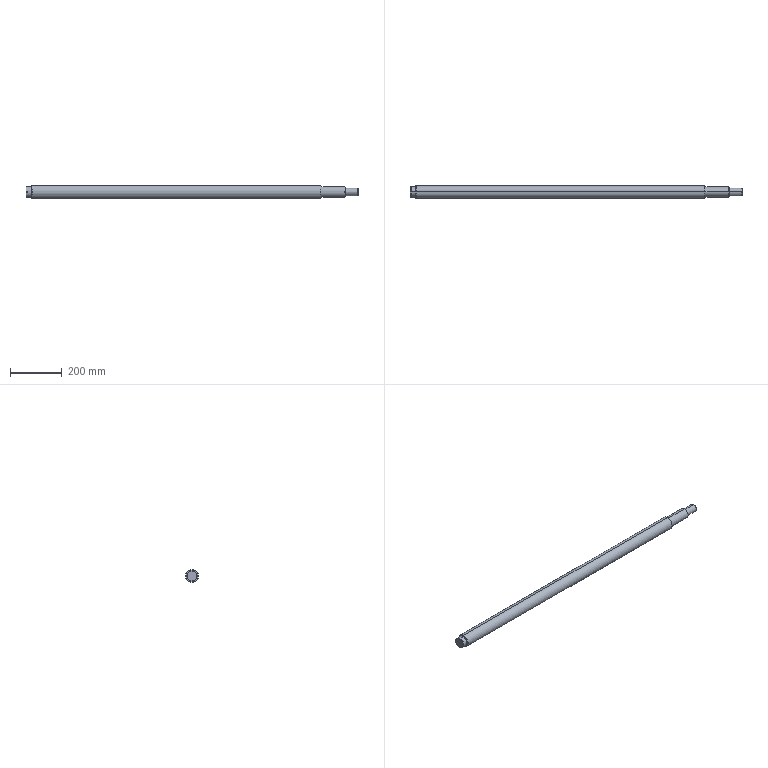Part | SolidWorks | features RefAxis 6, 3DProfileFeature 2, ICE 1, LockFeature 1, Revolution 1 | 1 solid | 36 faces | box 1281 x 50 x 50 mm | volume 2368676 mm3 | cylinder 14 | cone 10 | plane 10 | torus 2 | commonest cylinder face diameters 40 x6 8 x2 30 x2 38 x2 50 x2
STEP:
#1=CARTESIAN_POINT('',(0.,0.,19.));
#2=VERTEX_POINT('',#1);
#3=CARTESIAN_POINT('',(0.,0.,-19.));
#4=VERTEX_POINT('',#3);
#5=CARTESIAN_POINT('',(0.,0.,0.));
#6=DIRECTION('',(-1.,0.,0.));
#7=DIRECTION('',(0.,0.,1.));
#8=AXIS2_PLACEMENT_3D('',#5,#6,#7);
#9=CIRCLE('',#8,19.);
#10=EDGE_CURVE('',#2,#4,#9,.T.);
#11=ORIENTED_EDGE('',*,*,#10,.F.);
#12=CARTESIAN_POINT('',(1.,0.,20.));
#13=VERTEX_POINT('',#12);
#14=CARTESIAN_POINT('',(1.,0.,20.));
#15=DIRECTION('',(0.7071,0.,0.7071));
#16=VECTOR('',#15,1000.);
#17=LINE('',#14,#16);
#18=EDGE_CURVE('',#2,#13,#17,.T.);
#19=ORIENTED_EDGE('',*,*,#18,.T.);
#20=CARTESIAN_POINT('',(1.,0.,-20.));
#21=VERTEX_POINT('',#20);
#22=CARTESIAN_POINT('',(1.,0.,0.));
#23=DIRECTION('',(-1.,0.,0.));
#24=DIRECTION('',(0.,0.,1.));
#25=AXIS2_PLACEMENT_3D('',#22,#23,#24);
#26=CIRCLE('',#25,20.);
#27=EDGE_CURVE('',#13,#21,#26,.T.);
#28=ORIENTED_EDGE('',*,*,#27,.T.);
#29=CARTESIAN_POINT('',(1.,0.,-20.));
#30=DIRECTION('',(0.7071,0.,-0.7071));
#31=VECTOR('',#30,1000.);
#32=LINE('',#29,#31);
#33=EDGE_CURVE('',#4,#21,#32,.T.);
#34=ORIENTED_EDGE('',*,*,#33,.F.);
#35=EDGE_LOOP('',(#11,#19,#28,#34));
#36=FACE_OUTER_BOUND('',#35,.T.);
#37=CARTESIAN_POINT('',(1.,0.,0.));
#38=DIRECTION('',(1.,0.,0.));
#39=DIRECTION('',(0.,0.,-1.));
#40=AXIS2_PLACEMENT_3D('',#37,#38,#39);
#41=CONICAL_SURFACE('',#40,20.,0.7854);
#42=ADVANCED_FACE('',(#36),#41,.T.);
#43=CARTESIAN_POINT('',(3.05,0.,20.));
#44=VERTEX_POINT('',#43);
#45=CARTESIAN_POINT('',(3.05,0.,-20.));
#46=VERTEX_POINT('',#45);
#47=CARTESIAN_POINT('',(3.05,0.,0.));
#48=DIRECTION('',(-1.,0.,0.));
#49=DIRECTION('',(0.,0.,1.));
#50=AXIS2_PLACEMENT_3D('',#47,#48,#49);
#51=CIRCLE('',#50,20.);
#52=EDGE_CURVE('',#44,#46,#51,.T.);
#53=ORIENTED_EDGE('',*,*,#52,.T.);
#54=CARTESIAN_POINT('',(1281.,0.,-20.));
#55=DIRECTION('',(-1.,0.,0.));
#56=VECTOR('',#55,1000.);
#57=LINE('',#54,#56);
#58=EDGE_CURVE('',#46,#21,#57,.T.);
#59=ORIENTED_EDGE('',*,*,#58,.T.);
#60=ORIENTED_EDGE('',*,*,#27,.F.);
#61=CARTESIAN_POINT('',(1281.,0.,20.));
#62=DIRECTION('',(-1.,0.,0.));
#63=VECTOR('',#62,1000.);
#64=LINE('',#61,#63);
#65=EDGE_CURVE('',#44,#13,#64,.T.);
#66=ORIENTED_EDGE('',*,*,#65,.F.);
#67=EDGE_LOOP('',(#53,#59,#60,#66));
#68=FACE_OUTER_BOUND('',#67,.T.);
#69=CARTESIAN_POINT('',(1281.,0.,0.));
#70=DIRECTION('',(-1.,0.,0.));
#71=DIRECTION('',(0.,0.,1.));
#72=AXIS2_PLACEMENT_3D('',#69,#70,#71);
#73=CYLINDRICAL_SURFACE('',#72,20.);
#74=ADVANCED_FACE('',(#68),#73,.T.);
#75=CARTESIAN_POINT('',(5.,0.,19.));
#76=VERTEX_POINT('',#75);
#77=CARTESIAN_POINT('',(5.,0.,-19.));
#78=VERTEX_POINT('',#77);
#79=CARTESIAN_POINT('',(5.,0.,0.));
#80=DIRECTION('',(-1.,0.,0.));
#81=DIRECTION('',(0.,0.,1.));
#82=AXIS2_PLACEMENT_3D('',#79,#80,#81);
#83=CIRCLE('',#82,19.);
#84=EDGE_CURVE('',#76,#78,#83,.T.);
#85=ORIENTED_EDGE('',*,*,#84,.T.);
#86=CARTESIAN_POINT('',(3.05,0.,-19.));
#87=VERTEX_POINT('',#86);
#88=CARTESIAN_POINT('',(1281.,0.,-19.));
#89=DIRECTION('',(-1.,0.,0.));
#90=VECTOR('',#89,1000.);
#91=LINE('',#88,#90);
#92=EDGE_CURVE('',#78,#87,#91,.T.);
#93=ORIENTED_EDGE('',*,*,#92,.T.);
#94=CARTESIAN_POINT('',(3.05,0.,19.));
#95=VERTEX_POINT('',#94);
#96=CARTESIAN_POINT('',(3.05,0.,0.));
#97=DIRECTION('',(-1.,0.,0.));
#98=DIRECTION('',(0.,0.,1.));
#99=AXIS2_PLACEMENT_3D('',#96,#97,#98);
#100=CIRCLE('',#99,19.);
#101=EDGE_CURVE('',#95,#87,#100,.T.);
#102=ORIENTED_EDGE('',*,*,#101,.F.);
#103=CARTESIAN_POINT('',(1281.,0.,19.));
#104=DIRECTION('',(-1.,0.,0.));
#105=VECTOR('',#104,1000.);
#106=LINE('',#103,#105);
#107=EDGE_CURVE('',#76,#95,#106,.T.);
#108=ORIENTED_EDGE('',*,*,#107,.F.);
#109=EDGE_LOOP('',(#85,#93,#102,#108));
#110=FACE_OUTER_BOUND('',#109,.T.);
#111=CARTESIAN_POINT('',(1281.,0.,0.));
#112=DIRECTION('',(-1.,0.,0.));
#113=DIRECTION('',(0.,0.,1.));
#114=AXIS2_PLACEMENT_3D('',#111,#112,#113);
#115=CYLINDRICAL_SURFACE('',#114,19.);
#116=ADVANCED_FACE('',(#110),#115,.T.);
#117=CARTESIAN_POINT('',(22.75,0.,20.));
#118=VERTEX_POINT('',#117);
#119=CARTESIAN_POINT('',(22.75,0.,-20.));
#120=VERTEX_POINT('',#119);
#121=CARTESIAN_POINT('',(22.75,0.,0.));
#122=DIRECTION('',(-1.,0.,0.));
#123=DIRECTION('',(0.,0.,1.));
#124=AXIS2_PLACEMENT_3D('',#121,#122,#123);
#125=CIRCLE('',#124,20.);
#126=EDGE_CURVE('',#118,#120,#125,.T.);
#127=ORIENTED_EDGE('',*,*,#126,.T.);
#128=CARTESIAN_POINT('',(5.,0.,-20.));
#129=VERTEX_POINT('',#128);
#130=CARTESIAN_POINT('',(1281.,0.,-20.));
#131=DIRECTION('',(-1.,0.,0.));
#132=VECTOR('',#131,1000.);
#133=LINE('',#130,#132);
#134=EDGE_CURVE('',#120,#129,#133,.T.);
#135=ORIENTED_EDGE('',*,*,#134,.T.);
#136=CARTESIAN_POINT('',(5.,0.,20.));
#137=VERTEX_POINT('',#136);
#138=CARTESIAN_POINT('',(5.,0.,0.));
#139=DIRECTION('',(-1.,0.,0.));
#140=DIRECTION('',(0.,0.,1.));
#141=AXIS2_PLACEMENT_3D('',#138,#139,#140);
#142=CIRCLE('',#141,20.);
#143=EDGE_CURVE('',#137,#129,#142,.T.);
#144=ORIENTED_EDGE('',*,*,#143,.F.);
#145=CARTESIAN_POINT('',(1281.,0.,20.));
#146=DIRECTION('',(-1.,0.,0.));
#147=VECTOR('',#146,1000.);
#148=LINE('',#145,#147);
#149=EDGE_CURVE('',#118,#137,#148,.T.);
#150=ORIENTED_EDGE('',*,*,#149,.F.);
#151=EDGE_LOOP('',(#127,#135,#144,#150));
#152=FACE_OUTER_BOUND('',#151,.T.);
#153=CARTESIAN_POINT('',(1281.,0.,0.));
#154=DIRECTION('',(-1.,0.,0.));
#155=DIRECTION('',(0.,0.,1.));
#156=AXIS2_PLACEMENT_3D('',#153,#154,#155);
#157=CYLINDRICAL_SURFACE('',#156,20.);
#158=ADVANCED_FACE('',(#152),#157,.T.);
#159=CARTESIAN_POINT('',(22.75,0.,0.));
#160=DIRECTION('',(-1.,0.,0.));
#161=DIRECTION('',(0.,0.,1.));
#162=AXIS2_PLACEMENT_3D('',#159,#160,#161);
#163=CIRCLE('',#162,20.);
#164=EDGE_CURVE('',#120,#118,#163,.T.);
#165=ORIENTED_EDGE('',*,*,#164,.F.);
#166=CARTESIAN_POINT('',(23.,0.,-20.25));
#167=VERTEX_POINT('',#166);
#168=CARTESIAN_POINT('',(22.75,0.,-20.25));
#169=DIRECTION('',(0.,1.,0.));
#170=DIRECTION('',(0.,0.,1.));
#171=AXIS2_PLACEMENT_3D('',#168,#169,#170);
#172=CIRCLE('',#171,0.25);
#173=EDGE_CURVE('',#120,#167,#172,.T.);
#174=ORIENTED_EDGE('',*,*,#173,.T.);
#175=CARTESIAN_POINT('',(23.,0.,20.25));
#176=VERTEX_POINT('',#175);
#177=CARTESIAN_POINT('',(23.,0.,0.));
#178=DIRECTION('',(-1.,0.,0.));
#179=DIRECTION('',(0.,0.,1.));
#180=AXIS2_PLACEMENT_3D('',#177,#178,#179);
#181=CIRCLE('',#180,20.25);
#182=EDGE_CURVE('',#167,#176,#181,.T.);
#183=ORIENTED_EDGE('',*,*,#182,.T.);
#184=CARTESIAN_POINT('',(22.75,0.,20.25));
#185=DIRECTION('',(0.,-1.,0.));
#186=DIRECTION('',(0.,0.,-1.));
#187=AXIS2_PLACEMENT_3D('',#184,#185,#186);
#188=CIRCLE('',#187,0.25);
#189=EDGE_CURVE('',#118,#176,#188,.T.);
#190=ORIENTED_EDGE('',*,*,#189,.F.);
#191=EDGE_LOOP('',(#165,#174,#183,#190));
#192=FACE_OUTER_BOUND('',#191,.T.);
#193=CARTESIAN_POINT('',(22.75,0.,0.));
#194=DIRECTION('',(-1.,0.,0.));
#195=DIRECTION('',(0.,0.,1.));
#196=AXIS2_PLACEMENT_3D('',#193,#194,#195);
#197=TOROIDAL_SURFACE('',#196,20.25,0.25);
#198=ADVANCED_FACE('',(#192),#197,.F.);
#199=CARTESIAN_POINT('',(23.,0.,24.));
#200=VERTEX_POINT('',#199);
#201=CARTESIAN_POINT('',(23.,0.,-24.));
#202=VERTEX_POINT('',#201);
#203=CARTESIAN_POINT('',(23.,0.,0.));
#204=DIRECTION('',(-1.,0.,0.));
#205=DIRECTION('',(0.,0.,1.));
#206=AXIS2_PLACEMENT_3D('',#203,#204,#205);
#207=CIRCLE('',#206,24.);
#208=EDGE_CURVE('',#200,#202,#207,.T.);
#209=ORIENTED_EDGE('',*,*,#208,.F.);
#210=CARTESIAN_POINT('',(24.,0.,25.));
#211=VERTEX_POINT('',#210);
#212=CARTESIAN_POINT('',(24.,0.,25.));
#213=DIRECTION('',(0.7071,0.,0.7071));
#214=VECTOR('',#213,1000.);
#215=LINE('',#212,#214);
#216=EDGE_CURVE('',#200,#211,#215,.T.);
#217=ORIENTED_EDGE('',*,*,#216,.T.);
#218=CARTESIAN_POINT('',(24.,0.,-25.));
#219=VERTEX_POINT('',#218);
#220=CARTESIAN_POINT('',(24.,0.,0.));
#221=DIRECTION('',(-1.,0.,0.));
#222=DIRECTION('',(0.,0.,1.));
#223=AXIS2_PLACEMENT_3D('',#220,#221,#222);
#224=CIRCLE('',#223,25.);
#225=EDGE_CURVE('',#211,#219,#224,.T.);
#226=ORIENTED_EDGE('',*,*,#225,.T.);
#227=CARTESIAN_POINT('',(24.,0.,-25.));
#228=DIRECTION('',(0.7071,0.,-0.7071));
#229=VECTOR('',#228,1000.);
#230=LINE('',#227,#229);
#231=EDGE_CURVE('',#202,#219,#230,.T.);
#232=ORIENTED_EDGE('',*,*,#231,.F.);
#233=EDGE_LOOP('',(#209,#217,#226,#232));
#234=FACE_OUTER_BOUND('',#233,.T.);
#235=CARTESIAN_POINT('',(24.,0.,0.));
#236=DIRECTION('',(1.,0.,0.));
#237=DIRECTION('',(0.,0.,-1.));
#238=AXIS2_PLACEMENT_3D('',#235,#236,#237);
#239=CONICAL_SURFACE('',#238,25.,0.7854);
#240=ADVANCED_FACE('',(#234),#239,.T.);
#241=CARTESIAN_POINT('',(1137.,0.,25.));
#242=VERTEX_POINT('',#241);
#243=CARTESIAN_POINT('',(1137.,0.,-25.));
#244=VERTEX_POINT('',#243);
#245=CARTESIAN_POINT('',(1137.,0.,0.));
#246=DIRECTION('',(-1.,0.,0.));
#247=DIRECTION('',(0.,0.,1.));
#248=AXIS2_PLACEMENT_3D('',#245,#246,#247);
#249=CIRCLE('',#248,25.);
#250=EDGE_CURVE('',#242,#244,#249,.T.);
#251=ORIENTED_EDGE('',*,*,#250,.T.);
#252=CARTESIAN_POINT('',(1281.,0.,-25.));
#253=DIRECTION('',(-1.,0.,0.));
#254=VECTOR('',#253,1000.);
#255=LINE('',#252,#254);
#256=EDGE_CURVE('',#244,#219,#255,.T.);
#257=ORIENTED_EDGE('',*,*,#256,.T.);
#258=ORIENTED_EDGE('',*,*,#225,.F.);
#259=CARTESIAN_POINT('',(1281.,0.,25.));
#260=DIRECTION('',(-1.,0.,0.));
#261=VECTOR('',#260,1000.);
#262=LINE('',#259,#261);
#263=EDGE_CURVE('',#242,#211,#262,.T.);
#264=ORIENTED_EDGE('',*,*,#263,.F.);
#265=EDGE_LOOP('',(#251,#257,#258,#264));
#266=FACE_OUTER_BOUND('',#265,.T.);
#267=CARTESIAN_POINT('',(1281.,0.,0.));
#268=DIRECTION('',(-1.,0.,0.));
#269=DIRECTION('',(0.,0.,1.));
#270=AXIS2_PLACEMENT_3D('',#267,#268,#269);
#271=CYLINDRICAL_SURFACE('',#270,25.);
#272=ADVANCED_FACE('',(#266),#271,.T.);
#273=CARTESIAN_POINT('',(1138.,0.,24.));
#274=VERTEX_POINT('',#273);
#275=CARTESIAN_POINT('',(1138.,0.,-24.));
#276=VERTEX_POINT('',#275);
#277=CARTESIAN_POINT('',(1138.,0.,0.));
#278=DIRECTION('',(-1.,0.,0.));
#279=DIRECTION('',(0.,0.,1.));
#280=AXIS2_PLACEMENT_3D('',#277,#278,#279);
#281=CIRCLE('',#280,24.);
#282=EDGE_CURVE('',#274,#276,#281,.T.);
#283=ORIENTED_EDGE('',*,*,#282,.T.);
#284=CARTESIAN_POINT('',(1138.,0.,-24.));
#285=DIRECTION('',(-0.7071,0.,-0.7071));
#286=VECTOR('',#285,1000.);
#287=LINE('',#284,#286);
#288=EDGE_CURVE('',#276,#244,#287,.T.);
#289=ORIENTED_EDGE('',*,*,#288,.T.);
#290=ORIENTED_EDGE('',*,*,#250,.F.);
#291=CARTESIAN_POINT('',(1138.,0.,24.));
#292=DIRECTION('',(-0.7071,0.,0.7071));
#293=VECTOR('',#292,1000.);
#294=LINE('',#291,#293);
#295=EDGE_CURVE('',#274,#242,#294,.T.);
#296=ORIENTED_EDGE('',*,*,#295,.F.);
#297=EDGE_LOOP('',(#283,#289,#290,#296));
#298=FACE_OUTER_BOUND('',#297,.T.);
#299=CARTESIAN_POINT('',(1138.,0.,0.));
#300=DIRECTION('',(-1.,0.,0.));
#301=DIRECTION('',(0.,0.,1.));
#302=AXIS2_PLACEMENT_3D('',#299,#300,#301);
#303=CONICAL_SURFACE('',#302,24.,0.7854);
#304=ADVANCED_FACE('',(#298),#303,.T.);
#305=CARTESIAN_POINT('',(1230.,0.,20.));
#306=VERTEX_POINT('',#305);
#307=CARTESIAN_POINT('',(1230.,0.,-20.));
#308=VERTEX_POINT('',#307);
#309=CARTESIAN_POINT('',(1230.,0.,0.));
#310=DIRECTION('',(-1.,0.,0.));
#311=DIRECTION('',(0.,0.,1.));
#312=AXIS2_PLACEMENT_3D('',#309,#310,#311);
#313=CIRCLE('',#312,20.);
#314=EDGE_CURVE('',#306,#308,#313,.T.);
#315=ORIENTED_EDGE('',*,*,#314,.T.);
#316=CARTESIAN_POINT('',(1138.,0.,-20.));
#317=VERTEX_POINT('',#316);
#318=CARTESIAN_POINT('',(1281.,0.,-20.));
#319=DIRECTION('',(-1.,0.,0.));
#320=VECTOR('',#319,1000.);
#321=LINE('',#318,#320);
#322=EDGE_CURVE('',#308,#317,#321,.T.);
#323=ORIENTED_EDGE('',*,*,#322,.T.);
#324=CARTESIAN_POINT('',(1138.,0.,20.));
#325=VERTEX_POINT('',#324);
#326=CARTESIAN_POINT('',(1138.,0.,0.));
#327=DIRECTION('',(-1.,0.,0.));
#328=DIRECTION('',(0.,0.,1.));
#329=AXIS2_PLACEMENT_3D('',#326,#327,#328);
#330=CIRCLE('',#329,20.);
#331=EDGE_CURVE('',#325,#317,#330,.T.);
#332=ORIENTED_EDGE('',*,*,#331,.F.);
#333=CARTESIAN_POINT('',(1281.,0.,20.));
#334=DIRECTION('',(-1.,0.,0.));
#335=VECTOR('',#334,1000.);
#336=LINE('',#333,#335);
#337=EDGE_CURVE('',#306,#325,#336,.T.);
#338=ORIENTED_EDGE('',*,*,#337,.F.);
#339=EDGE_LOOP('',(#315,#323,#332,#338));
#340=FACE_OUTER_BOUND('',#339,.T.);
#341=CARTESIAN_POINT('',(1281.,0.,0.));
#342=DIRECTION('',(-1.,0.,0.));
#343=DIRECTION('',(0.,0.,1.));
#344=AXIS2_PLACEMENT_3D('',#341,#342,#343);
#345=CYLINDRICAL_SURFACE('',#344,20.);
#346=ADVANCED_FACE('',(#340),#345,.T.);
#347=CARTESIAN_POINT('',(1231.,0.,19.));
#348=VERTEX_POINT('',#347);
#349=CARTESIAN_POINT('',(1231.,0.,-19.));
#350=VERTEX_POINT('',#349);
#351=CARTESIAN_POINT('',(1231.,0.,0.));
#352=DIRECTION('',(-1.,0.,0.));
#353=DIRECTION('',(0.,0.,1.));
#354=AXIS2_PLACEMENT_3D('',#351,#352,#353);
#355=CIRCLE('',#354,19.);
#356=EDGE_CURVE('',#348,#350,#355,.T.);
#357=ORIENTED_EDGE('',*,*,#356,.T.);
#358=CARTESIAN_POINT('',(1231.,0.,-19.));
#359=DIRECTION('',(-0.7071,0.,-0.7071));
#360=VECTOR('',#359,1000.);
#361=LINE('',#358,#360);
#362=EDGE_CURVE('',#350,#308,#361,.T.);
#363=ORIENTED_EDGE('',*,*,#362,.T.);
#364=ORIENTED_EDGE('',*,*,#314,.F.);
#365=CARTESIAN_POINT('',(1231.,0.,19.));
#366=DIRECTION('',(-0.7071,0.,0.7071));
#367=VECTOR('',#366,1000.);
#368=LINE('',#365,#367);
#369=EDGE_CURVE('',#348,#306,#368,.T.);
#370=ORIENTED_EDGE('',*,*,#369,.F.);
#371=EDGE_LOOP('',(#357,#363,#364,#370));
#372=FACE_OUTER_BOUND('',#371,.T.);
#373=CARTESIAN_POINT('',(1231.,0.,0.));
#374=DIRECTION('',(-1.,0.,0.));
#375=DIRECTION('',(0.,0.,1.));
#376=AXIS2_PLACEMENT_3D('',#373,#374,#375);
#377=CONICAL_SURFACE('',#376,19.,0.7854);
#378=ADVANCED_FACE('',(#372),#377,.T.);
#379=CARTESIAN_POINT('',(1240.,14.457,-4.));
#380=VERTEX_POINT('',#379);
#381=CARTESIAN_POINT('',(1272.,14.457,-4.));
#382=VERTEX_POINT('',#381);
#383=CARTESIAN_POINT('',(1281.,14.457,-4.));
#384=DIRECTION('',(1.,0.,0.));
#385=VECTOR('',#384,1000.);
#386=LINE('',#383,#385);
#387=EDGE_CURVE('',#380,#382,#386,.T.);
#388=ORIENTED_EDGE('',*,*,#387,.T.);
#389=CARTESIAN_POINT('',(1272.,14.457,4.));
#390=VERTEX_POINT('',#389);
#391=CARTESIAN_POINT('',(1272.,14.457,-4.));
#392=CARTESIAN_POINT('',(1272.266,14.457,-4.));
#393=CARTESIAN_POINT('',(1272.526,14.464,-3.974));
#394=CARTESIAN_POINT('',(1273.039,14.492,-3.872));
#395=CARTESIAN_POINT('',(1273.294,14.513,-3.794));
#396=CARTESIAN_POINT('',(1273.777,14.564,-3.593));
#397=CARTESIAN_POINT('',(1274.007,14.594,-3.47));
#398=CARTESIAN_POINT('',(1274.44,14.66,-3.18));
#399=CARTESIAN_POINT('',(1274.645,14.696,-3.012));
#400=CARTESIAN_POINT('',(1275.012,14.766,-2.645));
#401=CARTESIAN_POINT('',(1275.177,14.801,-2.444));
#402=CARTESIAN_POINT('',(1275.47,14.867,-2.008));
#403=CARTESIAN_POINT('',(1275.593,14.896,-1.777));
#404=CARTESIAN_POINT('',(1275.793,14.946,-1.296));
#405=CARTESIAN_POINT('',(1275.871,14.966,-1.043));
#406=CARTESIAN_POINT('',(1275.974,14.993,-0.5261));
#407=CARTESIAN_POINT('',(1276.,15.,-0.2658));
#408=CARTESIAN_POINT('',(1276.,15.,0.2585));
#409=CARTESIAN_POINT('',(1275.974,14.993,0.5249));
#410=CARTESIAN_POINT('',(1275.872,14.966,1.039));
#411=CARTESIAN_POINT('',(1275.796,14.947,1.289));
#412=CARTESIAN_POINT('',(1275.494,14.872,2.017));
#413=CARTESIAN_POINT('',(1275.199,14.802,2.457));
#414=CARTESIAN_POINT('',(1274.645,14.696,3.012));
#415=CARTESIAN_POINT('',(1274.444,14.66,3.177));
#416=CARTESIAN_POINT('',(1274.012,14.595,3.467));
#417=CARTESIAN_POINT('',(1273.778,14.564,3.593));
#418=CARTESIAN_POINT('',(1273.296,14.513,3.793));
#419=CARTESIAN_POINT('',(1273.046,14.492,3.87));
#420=CARTESIAN_POINT('',(1272.531,14.464,3.973));
#421=CARTESIAN_POINT('',(1272.266,14.457,4.));
#422=CARTESIAN_POINT('',(1272.,14.457,4.));
#423=B_SPLINE_CURVE_WITH_KNOTS('',3,(#391,#392,#393,#394,#395,#396,#397,#398,#399,#400,#401,#402,#403,#404,#405,#406,#407,#408,#409,#410,#411,#412,#413,#414,#415,#416,#417,#418,#419,#420,#421,#422),.UNSPECIFIED.,.F.,.F.,(4,2,2,2,2,2,2,2,2,2,2,2,2,2,2,4),(0.,0.0007849,0.00157,0.002355,0.00314,0.003925,0.00471,0.005494,0.006279,0.007064,0.007849,0.009419,0.0102,0.01099,0.01177,0.01256),.UNSPECIFIED.);
#424=EDGE_CURVE('',#382,#390,#423,.T.);
#425=ORIENTED_EDGE('',*,*,#424,.T.);
#426=CARTESIAN_POINT('',(1240.,14.457,4.));
#427=VERTEX_POINT('',#426);
#428=CARTESIAN_POINT('',(1281.,14.457,4.));
#429=DIRECTION('',(-1.,0.,0.));
#430=VECTOR('',#429,1000.);
#431=LINE('',#428,#430);
#432=EDGE_CURVE('',#390,#427,#431,.T.);
#433=ORIENTED_EDGE('',*,*,#432,.T.);
#434=CARTESIAN_POINT('',(1240.,14.457,4.));
#435=CARTESIAN_POINT('',(1239.734,14.457,4.));
#436=CARTESIAN_POINT('',(1239.474,14.464,3.974));
#437=CARTESIAN_POINT('',(1238.961,14.492,3.872));
#438=CARTESIAN_POINT('',(1238.706,14.513,3.794));
#439=CARTESIAN_POINT('',(1238.223,14.564,3.593));
#440=CARTESIAN_POINT('',(1237.993,14.594,3.47));
#441=CARTESIAN_POINT('',(1237.56,14.66,3.18));
#442=CARTESIAN_POINT('',(1237.355,14.696,3.012));
#443=CARTESIAN_POINT('',(1236.988,14.766,2.645));
#444=CARTESIAN_POINT('',(1236.823,14.801,2.444));
#445=CARTESIAN_POINT('',(1236.53,14.867,2.008));
#446=CARTESIAN_POINT('',(1236.407,14.896,1.777));
#447=CARTESIAN_POINT('',(1236.207,14.946,1.296));
#448=CARTESIAN_POINT('',(1236.129,14.966,1.043));
#449=CARTESIAN_POINT('',(1236.026,14.993,0.5261));
#450=CARTESIAN_POINT('',(1236.,15.,0.2658));
#451=CARTESIAN_POINT('',(1236.,15.,-0.2585));
#452=CARTESIAN_POINT('',(1236.026,14.993,-0.5249));
#453=CARTESIAN_POINT('',(1236.128,14.966,-1.039));
#454=CARTESIAN_POINT('',(1236.204,14.947,-1.289));
#455=CARTESIAN_POINT('',(1236.506,14.872,-2.017));
#456=CARTESIAN_POINT('',(1236.801,14.802,-2.457));
#457=CARTESIAN_POINT('',(1237.355,14.696,-3.012));
#458=CARTESIAN_POINT('',(1237.556,14.66,-3.177));
#459=CARTESIAN_POINT('',(1237.988,14.595,-3.467));
#460=CARTESIAN_POINT('',(1238.222,14.564,-3.593));
#461=CARTESIAN_POINT('',(1238.704,14.513,-3.793));
#462=CARTESIAN_POINT('',(1238.954,14.492,-3.87));
#463=CARTESIAN_POINT('',(1239.469,14.464,-3.973));
#464=CARTESIAN_POINT('',(1239.734,14.457,-4.));
#465=CARTESIAN_POINT('',(1240.,14.457,-4.));
#466=B_SPLINE_CURVE_WITH_KNOTS('',3,(#434,#435,#436,#437,#438,#439,#440,#441,#442,#443,#444,#445,#446,#447,#448,#449,#450,#451,#452,#453,#454,#455,#456,#457,#458,#459,#460,#461,#462,#463,#464,#465),.UNSPECIFIED.,.F.,.F.,(4,2,2,2,2,2,2,2,2,2,2,2,2,2,2,4),(0.,0.0007849,0.00157,0.002355,0.00314,0.003925,0.00471,0.005494,0.006279,0.007064,0.007849,0.009419,0.0102,0.01099,0.01177,0.01256),.UNSPECIFIED.);
#467=EDGE_CURVE('',#427,#380,#466,.T.);
#468=ORIENTED_EDGE('',*,*,#467,.T.);
#469=EDGE_LOOP('',(#388,#425,#433,#468));
#470=FACE_BOUND('',#469,.T.);
#471=CARTESIAN_POINT('',(1280.,0.,15.));
#472=VERTEX_POINT('',#471);
#473=CARTESIAN_POINT('',(1280.,0.,-15.));
#474=VERTEX_POINT('',#473);
#475=CARTESIAN_POINT('',(1280.,0.,0.));
#476=DIRECTION('',(-1.,0.,0.));
#477=DIRECTION('',(0.,0.,1.));
#478=AXIS2_PLACEMENT_3D('',#475,#476,#477);
#479=CIRCLE('',#478,15.);
#480=EDGE_CURVE('',#472,#474,#479,.T.);
#481=ORIENTED_EDGE('',*,*,#480,.T.);
#482=CARTESIAN_POINT('',(1231.,0.,-15.));
#483=VERTEX_POINT('',#482);
#484=CARTESIAN_POINT('',(1281.,0.,-15.));
#485=DIRECTION('',(-1.,0.,0.));
#486=VECTOR('',#485,1000.);
#487=LINE('',#484,#486);
#488=EDGE_CURVE('',#474,#483,#487,.T.);
#489=ORIENTED_EDGE('',*,*,#488,.T.);
#490=CARTESIAN_POINT('',(1231.,0.,15.));
#491=VERTEX_POINT('',#490);
#492=CARTESIAN_POINT('',(1231.,0.,0.));
#493=DIRECTION('',(-1.,0.,0.));
#494=DIRECTION('',(0.,0.,1.));
#495=AXIS2_PLACEMENT_3D('',#492,#493,#494);
#496=CIRCLE('',#495,15.);
#497=EDGE_CURVE('',#491,#483,#496,.T.);
#498=ORIENTED_EDGE('',*,*,#497,.F.);
#499=CARTESIAN_POINT('',(1281.,0.,15.));
#500=DIRECTION('',(-1.,0.,0.));
#501=VECTOR('',#500,1000.);
#502=LINE('',#499,#501);
#503=EDGE_CURVE('',#472,#491,#502,.T.);
#504=ORIENTED_EDGE('',*,*,#503,.F.);
#505=EDGE_LOOP('',(#481,#489,#498,#504));
#506=FACE_OUTER_BOUND('',#505,.T.);
#507=CARTESIAN_POINT('',(1281.,0.,0.));
#508=DIRECTION('',(-1.,0.,0.));
#509=DIRECTION('',(0.,0.,1.));
#510=AXIS2_PLACEMENT_3D('',#507,#508,#509);
#511=CYLINDRICAL_SURFACE('',#510,15.);
#512=ADVANCED_FACE('',(#470,#506),#511,.T.);
#513=CARTESIAN_POINT('',(1281.,0.,14.));
#514=VERTEX_POINT('',#513);
#515=CARTESIAN_POINT('',(1281.,0.,-14.));
#516=VERTEX_POINT('',#515);
#517=CARTESIAN_POINT('',(1281.,0.,0.));
#518=DIRECTION('',(-1.,0.,0.));
#519=DIRECTION('',(0.,0.,1.));
#520=AXIS2_PLACEMENT_3D('',#517,#518,#519);
#521=CIRCLE('',#520,14.);
#522=EDGE_CURVE('',#514,#516,#521,.T.);
#523=ORIENTED_EDGE('',*,*,#522,.T.);
#524=CARTESIAN_POINT('',(1281.,0.,-14.));
#525=DIRECTION('',(-0.7071,0.,-0.7071));
#526=VECTOR('',#525,1000.);
#527=LINE('',#524,#526);
#528=EDGE_CURVE('',#516,#474,#527,.T.);
#529=ORIENTED_EDGE('',*,*,#528,.T.);
#530=ORIENTED_EDGE('',*,*,#480,.F.);
#531=CARTESIAN_POINT('',(1281.,0.,14.));
#532=DIRECTION('',(-0.7071,0.,0.7071));
#533=VECTOR('',#532,1000.);
#534=LINE('',#531,#533);
#535=EDGE_CURVE('',#514,#472,#534,.T.);
#536=ORIENTED_EDGE('',*,*,#535,.F.);
#537=EDGE_LOOP('',(#523,#529,#530,#536));
#538=FACE_OUTER_BOUND('',#537,.T.);
#539=CARTESIAN_POINT('',(1281.,0.,0.));
#540=DIRECTION('',(-1.,0.,0.));
#541=DIRECTION('',(0.,0.,1.));
#542=AXIS2_PLACEMENT_3D('',#539,#540,#541);
#543=CONICAL_SURFACE('',#542,14.,0.7854);
#544=ADVANCED_FACE('',(#538),#543,.T.);
#545=ORIENTED_EDGE('',*,*,#522,.F.);
#546=CARTESIAN_POINT('',(1281.,0.,0.));
#547=DIRECTION('',(-1.,0.,0.));
#548=DIRECTION('',(0.,0.,1.));
#549=AXIS2_PLACEMENT_3D('',#546,#547,#548);
#550=CIRCLE('',#549,14.);
#551=EDGE_CURVE('',#516,#514,#550,.T.);
#552=ORIENTED_EDGE('',*,*,#551,.F.);
#553=EDGE_LOOP('',(#545,#552));
#554=FACE_OUTER_BOUND('',#553,.T.);
#555=CARTESIAN_POINT('',(1281.,14.,0.));
#556=DIRECTION('',(-1.,0.,0.));
#557=DIRECTION('',(0.,0.,1.));
#558=AXIS2_PLACEMENT_3D('',#555,#556,#557);
#559=PLANE('',#558);
#560=ADVANCED_FACE('',(#554),#559,.F.);
#561=ORIENTED_EDGE('',*,*,#528,.F.);
#562=ORIENTED_EDGE('',*,*,#551,.T.);
#563=ORIENTED_EDGE('',*,*,#535,.T.);
#564=CARTESIAN_POINT('',(1280.,0.,0.));
#565=DIRECTION('',(-1.,0.,0.));
#566=DIRECTION('',(0.,0.,1.));
#567=AXIS2_PLACEMENT_3D('',#564,#565,#566);
#568=CIRCLE('',#567,15.);
#569=EDGE_CURVE('',#474,#472,#568,.T.);
#570=ORIENTED_EDGE('',*,*,#569,.F.);
#571=EDGE_LOOP('',(#561,#562,#563,#570));
#572=FACE_OUTER_BOUND('',#571,.T.);
#573=CARTESIAN_POINT('',(1281.,0.,0.));
#574=DIRECTION('',(-1.,0.,0.));
#575=DIRECTION('',(0.,0.,1.));
#576=AXIS2_PLACEMENT_3D('',#573,#574,#575);
#577=CONICAL_SURFACE('',#576,14.,0.7854);
#578=ADVANCED_FACE('',(#572),#577,.T.);
#579=ORIENTED_EDGE('',*,*,#488,.F.);
#580=ORIENTED_EDGE('',*,*,#569,.T.);
#581=ORIENTED_EDGE('',*,*,#503,.T.);
#582=CARTESIAN_POINT('',(1231.,0.,0.));
#583=DIRECTION('',(-1.,0.,0.));
#584=DIRECTION('',(0.,0.,1.));
#585=AXIS2_PLACEMENT_3D('',#582,#583,#584);
#586=CIRCLE('',#585,15.);
#587=EDGE_CURVE('',#483,#491,#586,.T.);
#588=ORIENTED_EDGE('',*,*,#587,.F.);
#589=EDGE_LOOP('',(#579,#580,#581,#588));
#590=FACE_OUTER_BOUND('',#589,.T.);
#591=CARTESIAN_POINT('',(1281.,0.,0.));
#592=DIRECTION('',(-1.,0.,0.));
#593=DIRECTION('',(0.,0.,1.));
#594=AXIS2_PLACEMENT_3D('',#591,#592,#593);
#595=CYLINDRICAL_SURFACE('',#594,15.);
#596=ADVANCED_FACE('',(#590),#595,.T.);
#597=ORIENTED_EDGE('',*,*,#356,.F.);
#598=CARTESIAN_POINT('',(1231.,0.,0.));
#599=DIRECTION('',(-1.,0.,0.));
#600=DIRECTION('',(0.,0.,1.));
#601=AXIS2_PLACEMENT_3D('',#598,#599,#600);
#602=CIRCLE('',#601,19.);
#603=EDGE_CURVE('',#350,#348,#602,.T.);
#604=ORIENTED_EDGE('',*,*,#603,.F.);
#605=EDGE_LOOP('',(#597,#604));
#606=FACE_OUTER_BOUND('',#605,.T.);
#607=ORIENTED_EDGE('',*,*,#497,.T.);
#608=ORIENTED_EDGE('',*,*,#587,.T.);
#609=EDGE_LOOP('',(#607,#608));
#610=FACE_BOUND('',#609,.T.);
#611=CARTESIAN_POINT('',(1231.,19.,0.));
#612=DIRECTION('',(-1.,0.,0.));
#613=DIRECTION('',(0.,0.,1.));
#614=AXIS2_PLACEMENT_3D('',#611,#612,#613);
#615=PLANE('',#614);
#616=ADVANCED_FACE('',(#606,#610),#615,.F.);
#617=ORIENTED_EDGE('',*,*,#362,.F.);
#618=ORIENTED_EDGE('',*,*,#603,.T.);
#619=ORIENTED_EDGE('',*,*,#369,.T.);
#620=CARTESIAN_POINT('',(1230.,0.,0.));
#621=DIRECTION('',(-1.,0.,0.));
#622=DIRECTION('',(0.,0.,1.));
#623=AXIS2_PLACEMENT_3D('',#620,#621,#622);
#624=CIRCLE('',#623,20.);
#625=EDGE_CURVE('',#308,#306,#624,.T.);
#626=ORIENTED_EDGE('',*,*,#625,.F.);
#627=EDGE_LOOP('',(#617,#618,#619,#626));
#628=FACE_OUTER_BOUND('',#627,.T.);
#629=CARTESIAN_POINT('',(1231.,0.,0.));
#630=DIRECTION('',(-1.,0.,0.));
#631=DIRECTION('',(0.,0.,1.));
#632=AXIS2_PLACEMENT_3D('',#629,#630,#631);
#633=CONICAL_SURFACE('',#632,19.,0.7854);
#634=ADVANCED_FACE('',(#628),#633,.T.);
#635=ORIENTED_EDGE('',*,*,#322,.F.);
#636=ORIENTED_EDGE('',*,*,#625,.T.);
#637=ORIENTED_EDGE('',*,*,#337,.T.);
#638=CARTESIAN_POINT('',(1138.,0.,0.));
#639=DIRECTION('',(-1.,0.,0.));
#640=DIRECTION('',(0.,0.,1.));
#641=AXIS2_PLACEMENT_3D('',#638,#639,#640);
#642=CIRCLE('',#641,20.);
#643=EDGE_CURVE('',#317,#325,#642,.T.);
#644=ORIENTED_EDGE('',*,*,#643,.F.);
#645=EDGE_LOOP('',(#635,#636,#637,#644));
#646=FACE_OUTER_BOUND('',#645,.T.);
#647=CARTESIAN_POINT('',(1281.,0.,0.));
#648=DIRECTION('',(-1.,0.,0.));
#649=DIRECTION('',(0.,0.,1.));
#650=AXIS2_PLACEMENT_3D('',#647,#648,#649);
#651=CYLINDRICAL_SURFACE('',#650,20.);
#652=ADVANCED_FACE('',(#646),#651,.T.);
#653=ORIENTED_EDGE('',*,*,#282,.F.);
#654=CARTESIAN_POINT('',(1138.,0.,0.));
#655=DIRECTION('',(-1.,0.,0.));
#656=DIRECTION('',(0.,0.,1.));
#657=AXIS2_PLACEMENT_3D('',#654,#655,#656);
#658=CIRCLE('',#657,24.);
#659=EDGE_CURVE('',#276,#274,#658,.T.);
#660=ORIENTED_EDGE('',*,*,#659,.F.);
#661=EDGE_LOOP('',(#653,#660));
#662=FACE_OUTER_BOUND('',#661,.T.);
#663=ORIENTED_EDGE('',*,*,#331,.T.);
#664=ORIENTED_EDGE('',*,*,#643,.T.);
#665=EDGE_LOOP('',(#663,#664));
#666=FACE_BOUND('',#665,.T.);
#667=CARTESIAN_POINT('',(1138.,24.,0.));
#668=DIRECTION('',(-1.,0.,0.));
#669=DIRECTION('',(0.,0.,1.));
#670=AXIS2_PLACEMENT_3D('',#667,#668,#669);
#671=PLANE('',#670);
#672=ADVANCED_FACE('',(#662,#666),#671,.F.);
#673=ORIENTED_EDGE('',*,*,#288,.F.);
#674=ORIENTED_EDGE('',*,*,#659,.T.);
#675=ORIENTED_EDGE('',*,*,#295,.T.);
#676=CARTESIAN_POINT('',(1137.,0.,0.));
#677=DIRECTION('',(-1.,0.,0.));
#678=DIRECTION('',(0.,0.,1.));
#679=AXIS2_PLACEMENT_3D('',#676,#677,#678);
#680=CIRCLE('',#679,25.);
#681=EDGE_CURVE('',#244,#242,#680,.T.);
#682=ORIENTED_EDGE('',*,*,#681,.F.);
#683=EDGE_LOOP('',(#673,#674,#675,#682));
#684=FACE_OUTER_BOUND('',#683,.T.);
#685=CARTESIAN_POINT('',(1138.,0.,0.));
#686=DIRECTION('',(-1.,0.,0.));
#687=DIRECTION('',(0.,0.,1.));
#688=AXIS2_PLACEMENT_3D('',#685,#686,#687);
#689=CONICAL_SURFACE('',#688,24.,0.7854);
#690=ADVANCED_FACE('',(#684),#689,.T.);
#691=ORIENTED_EDGE('',*,*,#256,.F.);
#692=ORIENTED_EDGE('',*,*,#681,.T.);
#693=ORIENTED_EDGE('',*,*,#263,.T.);
#694=CARTESIAN_POINT('',(24.,0.,0.));
#695=DIRECTION('',(-1.,0.,0.));
#696=DIRECTION('',(0.,0.,1.));
#697=AXIS2_PLACEMENT_3D('',#694,#695,#696);
#698=CIRCLE('',#697,25.);
#699=EDGE_CURVE('',#219,#211,#698,.T.);
#700=ORIENTED_EDGE('',*,*,#699,.F.);
#701=EDGE_LOOP('',(#691,#692,#693,#700));
#702=FACE_OUTER_BOUND('',#701,.T.);
#703=CARTESIAN_POINT('',(1281.,0.,0.));
#704=DIRECTION('',(-1.,0.,0.));
#705=DIRECTION('',(0.,0.,1.));
#706=AXIS2_PLACEMENT_3D('',#703,#704,#705);
#707=CYLINDRICAL_SURFACE('',#706,25.);
#708=ADVANCED_FACE('',(#702),#707,.T.);
#709=ORIENTED_EDGE('',*,*,#216,.F.);
#710=CARTESIAN_POINT('',(23.,0.,0.));
#711=DIRECTION('',(-1.,0.,0.));
#712=DIRECTION('',(0.,0.,1.));
#713=AXIS2_PLACEMENT_3D('',#710,#711,#712);
#714=CIRCLE('',#713,24.);
#715=EDGE_CURVE('',#202,#200,#714,.T.);
#716=ORIENTED_EDGE('',*,*,#715,.F.);
#717=ORIENTED_EDGE('',*,*,#231,.T.);
#718=ORIENTED_EDGE('',*,*,#699,.T.);
#719=EDGE_LOOP('',(#709,#716,#717,#718));
#720=FACE_OUTER_BOUND('',#719,.T.);
#721=CARTESIAN_POINT('',(24.,0.,0.));
#722=DIRECTION('',(1.,0.,0.));
#723=DIRECTION('',(0.,0.,-1.));
#724=AXIS2_PLACEMENT_3D('',#721,#722,#723);
#725=CONICAL_SURFACE('',#724,25.,0.7854);
#726=ADVANCED_FACE('',(#720),#725,.T.);
#727=CARTESIAN_POINT('',(23.,0.,0.));
#728=DIRECTION('',(-1.,0.,0.));
#729=DIRECTION('',(0.,0.,1.));
#730=AXIS2_PLACEMENT_3D('',#727,#728,#729);
#731=CIRCLE('',#730,20.25);
#732=EDGE_CURVE('',#176,#167,#731,.T.);
#733=ORIENTED_EDGE('',*,*,#732,.F.);
#734=ORIENTED_EDGE('',*,*,#182,.F.);
#735=EDGE_LOOP('',(#733,#734));
#736=FACE_BOUND('',#735,.T.);
#737=ORIENTED_EDGE('',*,*,#715,.T.);
#738=ORIENTED_EDGE('',*,*,#208,.T.);
#739=EDGE_LOOP('',(#737,#738));
#740=FACE_OUTER_BOUND('',#739,.T.);
#741=CARTESIAN_POINT('',(23.,20.25,0.));
#742=DIRECTION('',(1.,0.,0.));
#743=DIRECTION('',(0.,0.,-1.));
#744=AXIS2_PLACEMENT_3D('',#741,#742,#743);
#745=PLANE('',#744);
#746=ADVANCED_FACE('',(#736,#740),#745,.F.);
#747=ORIENTED_EDGE('',*,*,#173,.F.);
#748=ORIENTED_EDGE('',*,*,#126,.F.);
#749=ORIENTED_EDGE('',*,*,#189,.T.);
#750=ORIENTED_EDGE('',*,*,#732,.T.);
#751=EDGE_LOOP('',(#747,#748,#749,#750));
#752=FACE_OUTER_BOUND('',#751,.T.);
#753=CARTESIAN_POINT('',(22.75,0.,0.));
#754=DIRECTION('',(-1.,0.,0.));
#755=DIRECTION('',(0.,0.,1.));
#756=AXIS2_PLACEMENT_3D('',#753,#754,#755);
#757=TOROIDAL_SURFACE('',#756,20.25,0.25);
#758=ADVANCED_FACE('',(#752),#757,.F.);
#759=ORIENTED_EDGE('',*,*,#134,.F.);
#760=ORIENTED_EDGE('',*,*,#164,.T.);
#761=ORIENTED_EDGE('',*,*,#149,.T.);
#762=CARTESIAN_POINT('',(5.,0.,0.));
#763=DIRECTION('',(-1.,0.,0.));
#764=DIRECTION('',(0.,0.,1.));
#765=AXIS2_PLACEMENT_3D('',#762,#763,#764);
#766=CIRCLE('',#765,20.);
#767=EDGE_CURVE('',#129,#137,#766,.T.);
#768=ORIENTED_EDGE('',*,*,#767,.F.);
#769=EDGE_LOOP('',(#759,#760,#761,#768));
#770=FACE_OUTER_BOUND('',#769,.T.);
#771=CARTESIAN_POINT('',(1281.,0.,0.));
#772=DIRECTION('',(-1.,0.,0.));
#773=DIRECTION('',(0.,0.,1.));
#774=AXIS2_PLACEMENT_3D('',#771,#772,#773);
#775=CYLINDRICAL_SURFACE('',#774,20.);
#776=ADVANCED_FACE('',(#770),#775,.T.);
#777=ORIENTED_EDGE('',*,*,#84,.F.);
#778=CARTESIAN_POINT('',(5.,0.,0.));
#779=DIRECTION('',(-1.,0.,0.));
#780=DIRECTION('',(0.,0.,1.));
#781=AXIS2_PLACEMENT_3D('',#778,#779,#780);
#782=CIRCLE('',#781,19.);
#783=EDGE_CURVE('',#78,#76,#782,.T.);
#784=ORIENTED_EDGE('',*,*,#783,.F.);
#785=EDGE_LOOP('',(#777,#784));
#786=FACE_BOUND('',#785,.T.);
#787=ORIENTED_EDGE('',*,*,#143,.T.);
#788=ORIENTED_EDGE('',*,*,#767,.T.);
#789=EDGE_LOOP('',(#787,#788));
#790=FACE_OUTER_BOUND('',#789,.T.);
#791=CARTESIAN_POINT('',(5.,19.,0.));
#792=DIRECTION('',(1.,0.,0.));
#793=DIRECTION('',(0.,0.,-1.));
#794=AXIS2_PLACEMENT_3D('',#791,#792,#793);
#795=PLANE('',#794);
#796=ADVANCED_FACE('',(#786,#790),#795,.F.);
#797=ORIENTED_EDGE('',*,*,#92,.F.);
#798=ORIENTED_EDGE('',*,*,#783,.T.);
#799=ORIENTED_EDGE('',*,*,#107,.T.);
#800=CARTESIAN_POINT('',(3.05,0.,0.));
#801=DIRECTION('',(-1.,0.,0.));
#802=DIRECTION('',(0.,0.,1.));
#803=AXIS2_PLACEMENT_3D('',#800,#801,#802);
#804=CIRCLE('',#803,19.);
#805=EDGE_CURVE('',#87,#95,#804,.T.);
#806=ORIENTED_EDGE('',*,*,#805,.F.);
#807=EDGE_LOOP('',(#797,#798,#799,#806));
#808=FACE_OUTER_BOUND('',#807,.T.);
#809=CARTESIAN_POINT('',(1281.,0.,0.));
#810=DIRECTION('',(-1.,0.,0.));
#811=DIRECTION('',(0.,0.,1.));
#812=AXIS2_PLACEMENT_3D('',#809,#810,#811);
#813=CYLINDRICAL_SURFACE('',#812,19.);
#814=ADVANCED_FACE('',(#808),#813,.T.);
#815=ORIENTED_EDGE('',*,*,#52,.F.);
#816=CARTESIAN_POINT('',(3.05,0.,0.));
#817=DIRECTION('',(-1.,0.,0.));
#818=DIRECTION('',(0.,0.,1.));
#819=AXIS2_PLACEMENT_3D('',#816,#817,#818);
#820=CIRCLE('',#819,20.);
#821=EDGE_CURVE('',#46,#44,#820,.T.);
#822=ORIENTED_EDGE('',*,*,#821,.F.);
#823=EDGE_LOOP('',(#815,#822));
#824=FACE_OUTER_BOUND('',#823,.T.);
#825=ORIENTED_EDGE('',*,*,#101,.T.);
#826=ORIENTED_EDGE('',*,*,#805,.T.);
#827=EDGE_LOOP('',(#825,#826));
#828=FACE_BOUND('',#827,.T.);
#829=CARTESIAN_POINT('',(3.05,20.,0.));
#830=DIRECTION('',(-1.,0.,0.));
#831=DIRECTION('',(0.,0.,1.));
#832=AXIS2_PLACEMENT_3D('',#829,#830,#831);
#833=PLANE('',#832);
#834=ADVANCED_FACE('',(#824,#828),#833,.F.);
#835=ORIENTED_EDGE('',*,*,#58,.F.);
#836=ORIENTED_EDGE('',*,*,#821,.T.);
#837=ORIENTED_EDGE('',*,*,#65,.T.);
#838=CARTESIAN_POINT('',(1.,0.,0.));
#839=DIRECTION('',(-1.,0.,0.));
#840=DIRECTION('',(0.,0.,1.));
#841=AXIS2_PLACEMENT_3D('',#838,#839,#840);
#842=CIRCLE('',#841,20.);
#843=EDGE_CURVE('',#21,#13,#842,.T.);
#844=ORIENTED_EDGE('',*,*,#843,.F.);
#845=EDGE_LOOP('',(#835,#836,#837,#844));
#846=FACE_OUTER_BOUND('',#845,.T.);
#847=CARTESIAN_POINT('',(1281.,0.,0.));
#848=DIRECTION('',(-1.,0.,0.));
#849=DIRECTION('',(0.,0.,1.));
#850=AXIS2_PLACEMENT_3D('',#847,#848,#849);
#851=CYLINDRICAL_SURFACE('',#850,20.);
#852=ADVANCED_FACE('',(#846),#851,.T.);
#853=ORIENTED_EDGE('',*,*,#18,.F.);
#854=CARTESIAN_POINT('',(0.,0.,0.));
#855=DIRECTION('',(-1.,0.,0.));
#856=DIRECTION('',(0.,0.,1.));
#857=AXIS2_PLACEMENT_3D('',#854,#855,#856);
#858=CIRCLE('',#857,19.);
#859=EDGE_CURVE('',#4,#2,#858,.T.);
#860=ORIENTED_EDGE('',*,*,#859,.F.);
#861=ORIENTED_EDGE('',*,*,#33,.T.);
#862=ORIENTED_EDGE('',*,*,#843,.T.);
#863=EDGE_LOOP('',(#853,#860,#861,#862));
#864=FACE_OUTER_BOUND('',#863,.T.);
#865=CARTESIAN_POINT('',(1.,0.,0.));
#866=DIRECTION('',(1.,0.,0.));
#867=DIRECTION('',(0.,0.,-1.));
#868=AXIS2_PLACEMENT_3D('',#865,#866,#867);
#869=CONICAL_SURFACE('',#868,20.,0.7854);
#870=ADVANCED_FACE('',(#864),#869,.T.);
#871=ORIENTED_EDGE('',*,*,#859,.T.);
#872=ORIENTED_EDGE('',*,*,#10,.T.);
#873=EDGE_LOOP('',(#871,#872));
#874=FACE_OUTER_BOUND('',#873,.T.);
#875=CARTESIAN_POINT('',(0.,0.,0.));
#876=DIRECTION('',(1.,0.,0.));
#877=DIRECTION('',(0.,0.,-1.));
#878=AXIS2_PLACEMENT_3D('',#875,#876,#877);
#879=PLANE('',#878);
#880=ADVANCED_FACE('',(#874),#879,.F.);
#881=CARTESIAN_POINT('',(1240.,11.,4.));
#882=VERTEX_POINT('',#881);
#883=CARTESIAN_POINT('',(1240.,11.,4.));
#884=DIRECTION('',(0.,1.,0.));
#885=VECTOR('',#884,1000.);
#886=LINE('',#883,#885);
#887=EDGE_CURVE('',#882,#427,#886,.T.);
#888=ORIENTED_EDGE('',*,*,#887,.F.);
#889=CARTESIAN_POINT('',(1240.,11.,-4.));
#890=VERTEX_POINT('',#889);
#891=CARTESIAN_POINT('',(1240.,11.,0.));
#892=DIRECTION('',(0.,1.,0.));
#893=DIRECTION('',(0.,0.,1.));
#894=AXIS2_PLACEMENT_3D('',#891,#892,#893);
#895=CIRCLE('',#894,4.);
#896=EDGE_CURVE('',#890,#882,#895,.T.);
#897=ORIENTED_EDGE('',*,*,#896,.F.);
#898=CARTESIAN_POINT('',(1240.,11.,-4.));
#899=DIRECTION('',(0.,1.,0.));
#900=VECTOR('',#899,1000.);
#901=LINE('',#898,#900);
#902=EDGE_CURVE('',#890,#380,#901,.T.);
#903=ORIENTED_EDGE('',*,*,#902,.T.);
#904=ORIENTED_EDGE('',*,*,#467,.F.);
#905=EDGE_LOOP('',(#888,#897,#903,#904));
#906=FACE_OUTER_BOUND('',#905,.T.);
#907=CARTESIAN_POINT('',(1240.,11.,0.));
#908=DIRECTION('',(0.,1.,0.));
#909=DIRECTION('',(0.,0.,1.));
#910=AXIS2_PLACEMENT_3D('',#907,#908,#909);
#911=CYLINDRICAL_SURFACE('',#910,4.);
#912=ADVANCED_FACE('',(#906),#911,.F.);
#913=ORIENTED_EDGE('',*,*,#902,.F.);
#914=CARTESIAN_POINT('',(1272.,11.,-4.));
#915=VERTEX_POINT('',#914);
#916=CARTESIAN_POINT('',(1272.,11.,-4.));
#917=DIRECTION('',(-1.,0.,0.));
#918=VECTOR('',#917,1000.);
#919=LINE('',#916,#918);
#920=EDGE_CURVE('',#915,#890,#919,.T.);
#921=ORIENTED_EDGE('',*,*,#920,.F.);
#922=CARTESIAN_POINT('',(1272.,11.,-4.));
#923=DIRECTION('',(0.,1.,0.));
#924=VECTOR('',#923,1000.);
#925=LINE('',#922,#924);
#926=EDGE_CURVE('',#915,#382,#925,.T.);
#927=ORIENTED_EDGE('',*,*,#926,.T.);
#928=ORIENTED_EDGE('',*,*,#387,.F.);
#929=EDGE_LOOP('',(#913,#921,#927,#928));
#930=FACE_OUTER_BOUND('',#929,.T.);
#931=CARTESIAN_POINT('',(1272.,11.,-4.));
#932=DIRECTION('',(0.,0.,-1.));
#933=DIRECTION('',(-1.,0.,0.));
#934=AXIS2_PLACEMENT_3D('',#931,#932,#933);
#935=PLANE('',#934);
#936=ADVANCED_FACE('',(#930),#935,.F.);
#937=ORIENTED_EDGE('',*,*,#926,.F.);
#938=CARTESIAN_POINT('',(1272.,11.,4.));
#939=VERTEX_POINT('',#938);
#940=CARTESIAN_POINT('',(1272.,11.,0.));
#941=DIRECTION('',(0.,1.,0.));
#942=DIRECTION('',(0.,0.,1.));
#943=AXIS2_PLACEMENT_3D('',#940,#941,#942);
#944=CIRCLE('',#943,4.);
#945=EDGE_CURVE('',#939,#915,#944,.T.);
#946=ORIENTED_EDGE('',*,*,#945,.F.);
#947=CARTESIAN_POINT('',(1272.,11.,4.));
#948=DIRECTION('',(0.,1.,0.));
#949=VECTOR('',#948,1000.);
#950=LINE('',#947,#949);
#951=EDGE_CURVE('',#939,#390,#950,.T.);
#952=ORIENTED_EDGE('',*,*,#951,.T.);
#953=ORIENTED_EDGE('',*,*,#424,.F.);
#954=EDGE_LOOP('',(#937,#946,#952,#953));
#955=FACE_OUTER_BOUND('',#954,.T.);
#956=CARTESIAN_POINT('',(1272.,11.,0.));
#957=DIRECTION('',(0.,1.,0.));
#958=DIRECTION('',(0.,0.,1.));
#959=AXIS2_PLACEMENT_3D('',#956,#957,#958);
#960=CYLINDRICAL_SURFACE('',#959,4.);
#961=ADVANCED_FACE('',(#955),#960,.F.);
#962=ORIENTED_EDGE('',*,*,#951,.F.);
#963=CARTESIAN_POINT('',(1240.,11.,4.));
#964=DIRECTION('',(1.,0.,0.));
#965=VECTOR('',#964,1000.);
#966=LINE('',#963,#965);
#967=EDGE_CURVE('',#882,#939,#966,.T.);
#968=ORIENTED_EDGE('',*,*,#967,.F.);
#969=ORIENTED_EDGE('',*,*,#887,.T.);
#970=ORIENTED_EDGE('',*,*,#432,.F.);
#971=EDGE_LOOP('',(#962,#968,#969,#970));
#972=FACE_OUTER_BOUND('',#971,.T.);
#973=CARTESIAN_POINT('',(1240.,11.,4.));
#974=DIRECTION('',(0.,0.,1.));
#975=DIRECTION('',(1.,0.,0.));
#976=AXIS2_PLACEMENT_3D('',#973,#974,#975);
#977=PLANE('',#976);
#978=ADVANCED_FACE('',(#972),#977,.F.);
#979=ORIENTED_EDGE('',*,*,#896,.T.);
#980=ORIENTED_EDGE('',*,*,#967,.T.);
#981=ORIENTED_EDGE('',*,*,#945,.T.);
#982=ORIENTED_EDGE('',*,*,#920,.T.);
#983=EDGE_LOOP('',(#979,#980,#981,#982));
#984=FACE_OUTER_BOUND('',#983,.T.);
#985=CARTESIAN_POINT('',(1240.,11.,0.));
#986=DIRECTION('',(0.,1.,0.));
#987=DIRECTION('',(0.,0.,1.));
#988=AXIS2_PLACEMENT_3D('',#985,#986,#987);
#989=PLANE('',#988);
#990=ADVANCED_FACE('',(#984),#989,.T.);
#991=CLOSED_SHELL('',(#42,#74,#116,#158,#198,#240,#272,#304,#346,#378,#512,#544,#560,#578,#596,#616,#634,#652,#672,#690,#708,#726,#746,#758,#776,#796,#814,#834,#852,#870,#880,#912,#936,#961,#978,#990));
#992=MANIFOLD_SOLID_BREP('',#991);
#993=CARTESIAN_POINT('',(0.,0.,0.));
#994=DIRECTION('',(0.,0.,1.));
#995=DIRECTION('',(1.,0.,0.));
#996=AXIS2_PLACEMENT_3D('',#993,#994,#995);
#997=(LENGTH_UNIT()NAMED_UNIT(*)SI_UNIT(.MILLI.,.METRE.));
#998=UNCERTAINTY_MEASURE_WITH_UNIT(LENGTH_MEASURE(0.00001),#997,'','');
#999=(NAMED_UNIT(*)PLANE_ANGLE_UNIT()SI_UNIT($,.RADIAN.));
#1000=(NAMED_UNIT(*)SI_UNIT($,.STERADIAN.)SOLID_ANGLE_UNIT());
#1001=(GEOMETRIC_REPRESENTATION_CONTEXT(3)GLOBAL_UNCERTAINTY_ASSIGNED_CONTEXT((#998))GLOBAL_UNIT_ASSIGNED_CONTEXT((#997,#999,#1000))REPRESENTATION_CONTEXT('',''));
#1002=ADVANCED_BREP_SHAPE_REPRESENTATION('',(#992,#996),#1001);